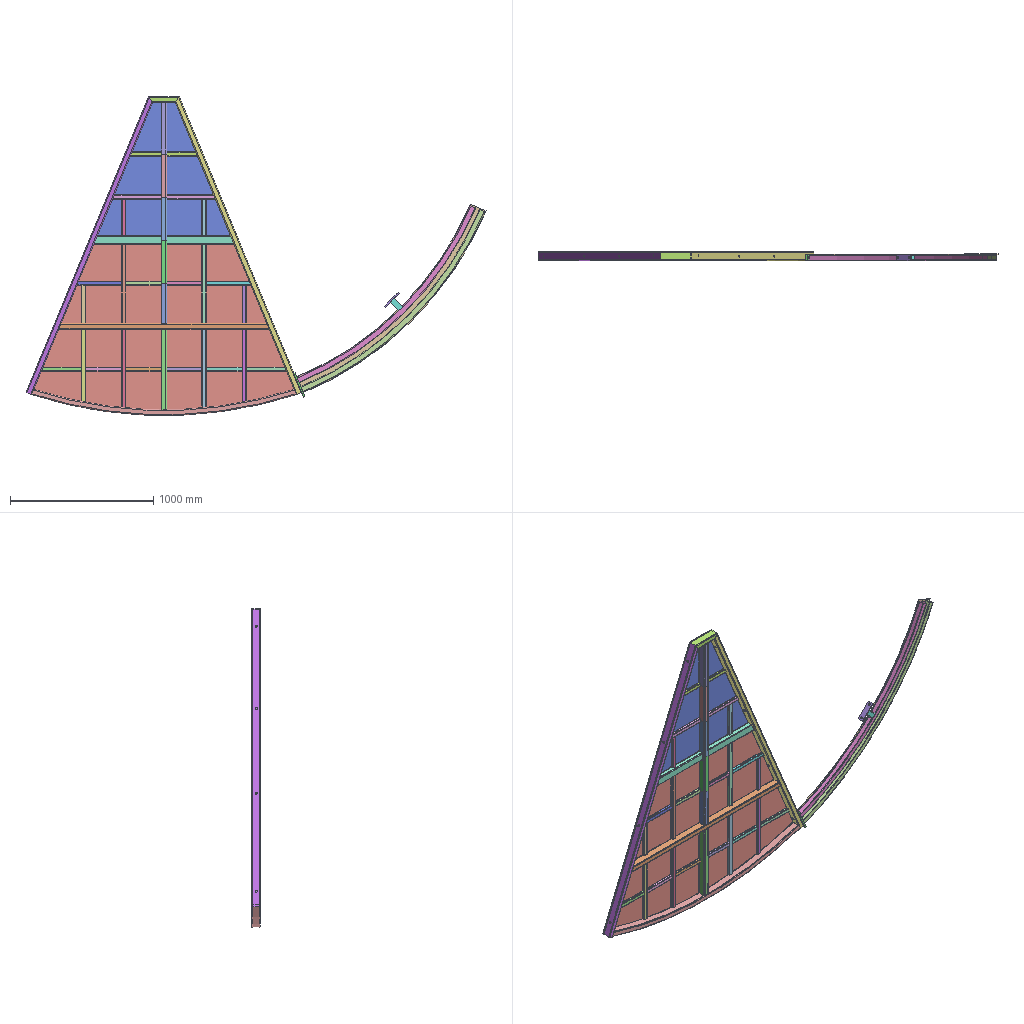Assembly | SolidWorks | 7 different items | 7 placed | box 3206 x 63 x 2221 mm
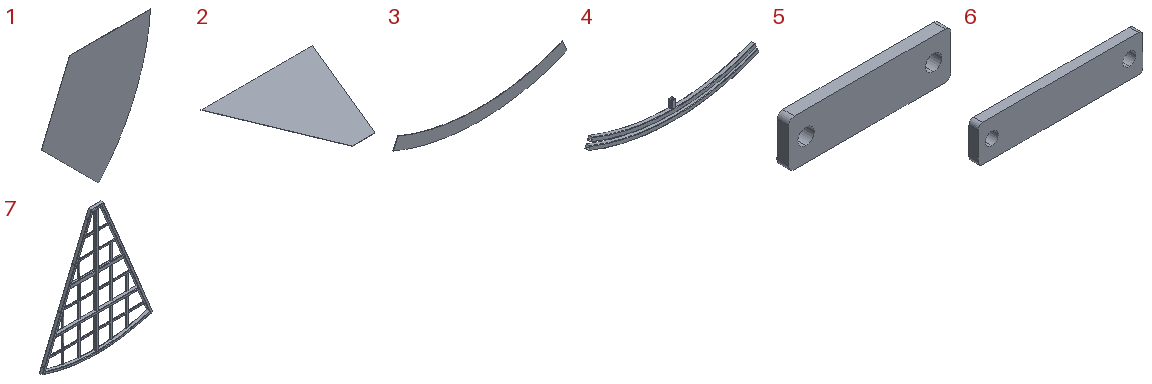Parts list (item | quantity | size | volume | features):
1 | x1 | 1549 x 2.5 x 1776 mm | 4445918 mm3 | features Extrusion 1
2 | x1 | 1042 x 1001 x 2.5 mm | 1569496 mm3 | features Extrusion 1
3 | x1 | 1806 x 5 x 290.423 mm | 1083568 mm3 | features Extrusion 1
4 | x1 | 1783 x 40 x 277.077 mm | 1072506 mm3 | features WeldCornerFeat 1, WeldMemberFeat 1, WeldmentFeature 1
5 | x1 | 140 x 10 x 40 mm | 52707 mm3 | features Extrusion 1
6 | x1 | 180 x 10 x 40 mm | 68707 mm3 | features Extrusion 1
7 | x1 | 1921 x 60 x 2222 mm | 7305764 mm3 | features WeldCornerFeat 13, WeldMemberFeat 5, HoleWzd 2, WeldmentFeature 1
Mates (type | each side: item.copy, entity, surface, feature):
Coincident | 4.1 face plane Cold-formed hollow square steel (gb t6728-2002) 40×2-example.com(1) | 6.1 face plane Boss-Extrude1 | 2 times
Coincident | 4.1 face plane Cold-formed hollow square steel (gb t6728-2002) 40×2-example.com(1) | 3.1 face plane Boss-Extrude1
Concentric | 4.1 face cylinder Cold-formed hollow square steel (gb t6728-2002) 40×2-example.com(1) | 3.1 face cylinder Boss-Extrude1
Coincident | 4.1 face plane Cold-formed hollow square steel (gb t6728-2002) 40×2-example.com(1) | 5.1 face plane Boss-Extrude1 | 2 times
DistanceDim | 3.1 face cylinder Boss-Extrude1 | 6.1 face plane Boss-Extrude1
Coincident | 7.1 face plane Cold-formed hollow rectangular steel (gb t6728-2002) 60×40×3(1) | 2.1 face plane Boss-Extrude1 | 2 times
Coincident | 7.1 face plane Cold-formed hollow rectangular steel (gb t6728-2002) 60×40×3(1) | 1.1 face plane Boss-Extrude2 | 2 times
Coincident | 1.1 face plane Boss-Extrude2 | 2.1 face plane Boss-Extrude1
Tangent | 7.1 face plane Cold-formed hollow rectangular steel (gb t6728-2002) 60×40×3(1) | 4.1 face cylinder Cold-formed hollow square steel (gb t6728-2002) 40×2-example.com(1)
Coincident | 7.1 face plane Cold-formed hollow rectangular steel (gb t6728-2002) 60×40×3(1) | 6.1 face plane Boss-Extrude1 | 2 times